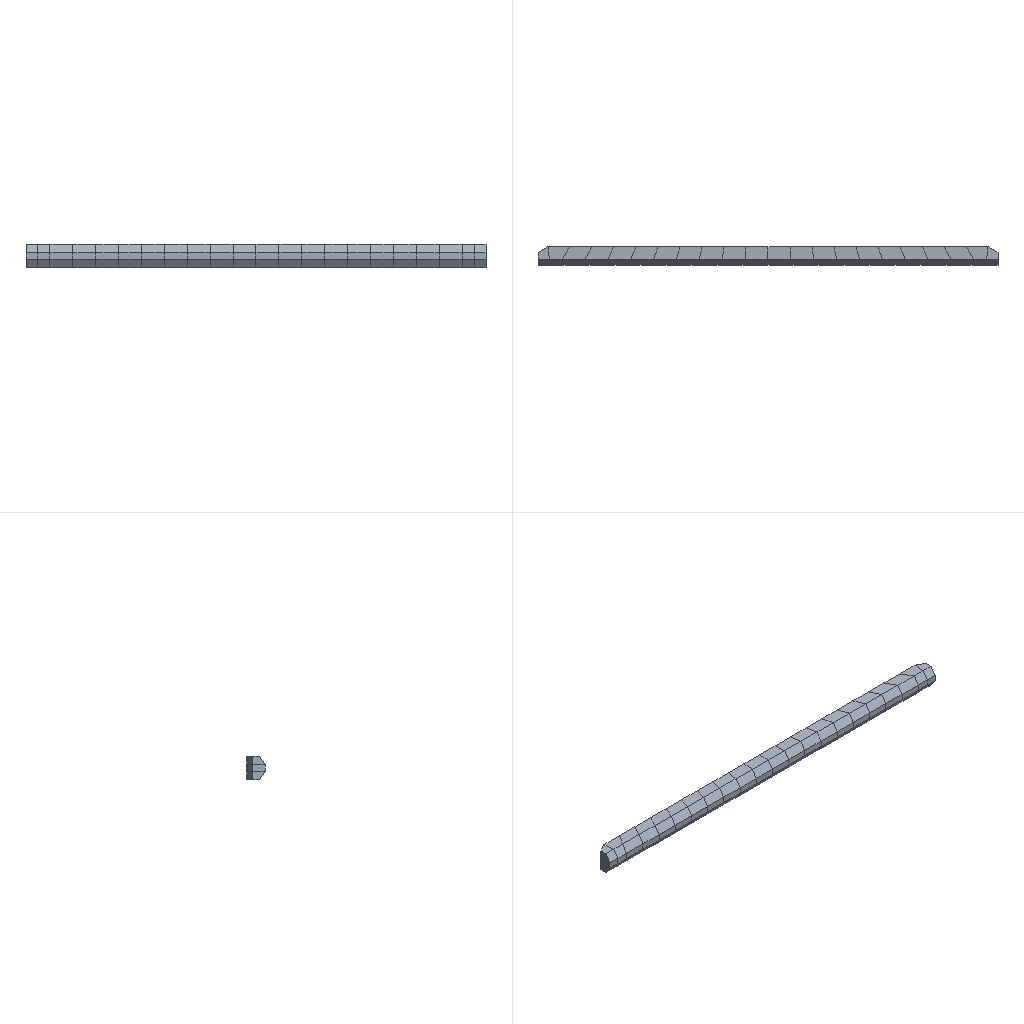Simulation study | ansys workbench
Set-up summary:
category,name,step,type,value,unit,region
solver,ansys_workbench
units,SI m-kg-s (Pa),,stated,"/units,MKS"
analysis,LS1,,static
load_step,LS1,LS1,static,nsubst=1; time=1
mesh,nodes,,,590
mesh,elements,,,126
element_type,SOLID186,,,66
element_type,SURF154,,,60
material,Q235B,,E,2e+11,Pa
material,Q235B,,nu,0.3
material,Q235B,,density,7850,kg m^-3
material,Q235B,,conductivity,60.5,W m^-1 C^-1
material,Q235B,,specific_heat,434,J kg^-1 C^-1
material,Q235B,,cte,1.2e-05,C^-1
material,Q235B,,permeability,10000
material,Q235B,,resistivity,1.7e-07,kg m^3 A^-2 s^-3
load,Define Force Using Surface Effect Elements,LS1,surface-effect pres face 2,-2613.15,,SURF154 #2
bc,Fixed Supports,model,fixed,[dofs=ALL],,_FIXEDSU
named_set,_FIXEDSU,,node,36
Ansys APDL input file, long lists of numbers shortened:
/batch
/config,noeldb,1     ! force off writing results to database
*get,_wallstrt,active,,time,wall
! ANSYS input file written by Workbench version 2022 R1
! File used for geometry attach:
/title,wbnew--____ (B5)
! ****** Begin Custom Load Command Snippet ******
/COM, ACT Extensions:
/COM,     LSDYNA, 2021.1
/COM,
! ****** End   Custom Load Command Snippet ******
*DIM,_wb_ProjectScratch_dir,string,248
_wb_ProjectScratch_dir(1) = ''
*DIM,_wb_SolverFiles_dir,string,248
_wb_SolverFiles_dir(1) = ''
*DIM,_wb_userfiles_dir,string,248
_wb_userfiles_dir(1) = ''
/com,--- Data in consistent MKS units. See Solving Units in the help system for more information.
/units,MKS
/nopr
/wb,file,start              !  signify a WB generated input file
/prep7
! Turn off shape checking because checks already performed inside WB mesher.
! See help system for more information.
SHPP,OFF,,NOWARN
/nolist
etcon,set             ! allow ANSYS to choose best KEYOP's for 180x elements, resets any applicable keyopt to MAPDL defaults
/com,*********** Nodes for the whole assembly ***********
nblock,3,,649
(1i9,3e20.9e3)
        1    -1.951259336E+01     1.555228924E-02     8.000000000E-01
! (589 more lines like these left out)
-1
/wb,elem,start            !  set before creation of elements
/com,*********** Elements for Body 1 "_-FreeParts|__2" ***********
et,1,186
keyo,1,2,1          ! set full integration on SOLID186
eblock,19,solid,,66
(19i9)
        1        1        1        1        0        0        0        0       20        0        1       70       71      123      120      114       93      122      121
! (131 more lines like these left out)
-1
/wb,elem,end               !  done creating elements
/com,*********** Send User Defined Coordinate System(s) ***********
csys,0
toffst,273.15,  ! Temperature offset from absolute zero
/com,*********** Set Reference Temperature ***********
tref,22.
/wb,mat,start              !  starting to send materials
/com,*********** Send Materials ***********
Temperature = 'TEMP' ! Temperature
MP,DENS,1,7850,	! kg m^-3
MP,ALPX,1,1.2e-05,	! C^-1
MP,C,1,434,	! J kg^-1 C^-1
MP,KXX,1,60.5,	! W m^-1 C^-1
MP,RSVX,1,1.7e-07,	! kg m^3 A^-2 s^-3
MP,EX,1,200000000000,	! Pa
MP,NUXY,1,0.3,
MP,MURX,1,10000,
/wb,mat,end                !  done sending materials
!************************* Model Summary ********************
!_-FreeParts|__2,	Q235B,	matid,	1
!************************* End Model Summary ********************
! get the diagonal of the bounding box. Needed later for other things
*get,_xmin,node,,mnloc,x
*get,_ymin,node,,mnloc,y
*get,_zmin,node,,mnloc,z
*get,_xmax,node,,mxloc,x
*get,_ymax,node,,mxloc,y
*get,_zmax,node,,mxloc,z
_ASMDIAG=(_xmax-_xmin)*(_xmax-_xmin)+(_ymax-_ymin)*(_ymax-_ymin)+(_zmax-_zmin)*(_zmax-_zmin)
_ASMDIAG=SQRT(_ASMDIAG)
/wb,contact,start          !  starting to send contact
/wb,contact,end            !  done creating contacts
/golist
/wb,load,start             !  starting to send loads
/com,*********** Fixed Supports ***********
CMBLOCK,_FIXEDSU,NODE,       36
(8i10)
        43        44        45        46        68        69        70        92
       114       115       116       117       118       119       120       121
       292       293       294       295       296       297       362       363
       364       365       367       368       432       433       477       478
       479       481       484       486
cmsel,s,_FIXEDSU
d,all,all
nsel,all
/com,*********** Define Force Using Surface Effect Elements ***********
local,12,0,0.,0.,0.,0.,0.,0.
csys,0
et,2,154
eblock,10,,,60
(15i9)
      249        2        2        2       12        2      125      182        1      191      496      188      185
! (59 more lines like these left out)
-1
esel,s,type,,2
keyop,2,2,1                ! Apply load in local coordinate system
keyop,2,7,1                ! Use original area so load is constant in large deformation
esel,all
/gst,on,on
fini
*get,_numnode,node,0,count
*get,_numelem,elem,0,count
*get, _MAXELEMNUM, elem, 0, NUM, MAX
*get, _MAXNODENUM, node, 0, NUM, MAX
*get, _MAXELEMTYPE, etyp, 0, NUM, MAX
*get, _MAXREALCONST, real, 0, NUM, MAX
/go
/wb,load,end               !  done creating loads
/com,--- Number of total nodes = %_numnode%
/com,--- Number of contact elements = 60
/com,--- Number of spring elements = 0
/com,--- Number of bearing elements = 0
/com,--- Number of solid elements = 66
/com,--- Number of condensed parts = 0
/com,--- Number of total elements = %_numelem%
*get,_wallbsol,active,,time,wall
/com,****************************************************************************
/com,*************************    SOLUTION       ********************************
/com,****************************************************************************
/solu
antype,0                   ! static analysis
_thickRatio=  0     ! Ratio of thick parts in the model
eqsl,sparse,,,,,1
cntr,print,1               ! print out contact info and also make no initial contact an error
dmpoption,emat,no             ! Don't combine emat file for DANSYS
dmpoption,esav,no             ! Don't combine esav file for DANSYS
nldiag,cont,iter           ! print out contact info each equilibrium iteration
rescontrol,,none                 ! Do not keep any restart files
/com,****************************************************
/com,******************* SOLVE FOR LS 1 OF 1 ****************
esel,s,type,,2
nsle
sfe,all,1,pres,1,0.
sfe,all,2,pres,1,-2613.153
sfe,all,3,pres,1,0.
nsel,all
esel,all
/nopr
/gopr
nsub,1,1,1
time,1.
outres,erase
outres,all,none
outres,nsol,all,
outres,rsol,all
outres,eangl,all
outres,etmp,all
outres,veng,all
outres,strs,all,
outres,epel,all,
outres,eppl,all,
outres,cont,all,
! *********** WB SOLVE COMMAND ***********
! check interactive state
*get,ANSINTER_,active,,int
*if,ANSINTER_,ne,0,then
/eof
*endif
solve
/com *************** Write FE CONNECTORS *********
CEWRITE,file,ce,,INTE
/com,****************************************************
/com,*************** FINISHED SOLVE FOR LS 1 *************
*get,_wallasol,active,,time,wall
/nopr
*get,_numnode,node,0,count
*get,_numelem,elem,0,count
*get, _MAXELEMNUM, elem, 0, NUM, MAX
*get, _MAXNODENUM, node, 0, NUM, MAX,,,INTERNAL
*get, _MAXELEMTYPE, etyp, 0, NUM, MAX
*get, _MAXREALCONST, real, 0, NUM, MAX
/gopr
/post1
xmlo,ENCODING,ISO-8859-1
xmlo,parm
/xml,parm,xml
fini
/gopr
*get,_walldone,active,,time,wall
_preptime=(_wallbsol-_wallstrt)*3600
_solvtime=(_wallasol-_wallbsol)*3600
_posttime=(_walldone-_wallasol)*3600
_totaltim=(_walldone-_wallstrt)*3600
*get,_dlbratio,active,0,solu,dlbr
*get,_combtime,active,0,solu,comb
*get,_ssmode,active,0,solu,ssmm
*get,_ndofs,active,0,solu,ndof
*get,_sol_end_time,active,0,set,time
*if,_sol_end_time,eq,1.,then
/fclean				!clean distributed files
*endif
/com,--- Total number of nodes = %_numnode%
/com,--- Total number of elements = %_numelem%
/com,--- Element load balance ratio = %_dlbratio%
/com,--- Time to combine distributed files = %_combtime%
/com,--- Sparse memory mode = %_ssmode%
/com,--- Number of DOF = %_ndofs%
/wb,file,end               ! done with WB generated input
Results summary:
result,analyses[0].index,,,1
result,analyses[0].system,,,SYS
result,analyses[0].deck,,,deck.dat
result,analyses[0].solve_status,,,completed
result,analyses[0].analysis_type,,,static
result,analyses[0].physics,,,mechanical
result,analyses[0].unit_system,,,"MKS: m, kg, N, s, V, A, degC"
result,analyses[0].n_sets,,,1
result,analyses[0].load_steps[0].set,set=1,,1
result,analyses[0].load_steps[0].time_or_freq,set=1,,1
result,analyses[0].load_steps[0].max_displacement_magnitude,set=1,,0.0001916
result,analyses[0].load_steps[0].max_von_mises_nodal,set=1,,1.57213e+06
result,analyses[0].load_steps[0].reaction_force_sum_xyz[1],set=1,,-1.32277e-08
result,analyses[0].load_steps[0].reaction_force_sum_xyz[2],set=1,,50000
result,analyses[0].load_steps[0].reaction_force_sum_xyz[3],set=1,,2.36812e-07